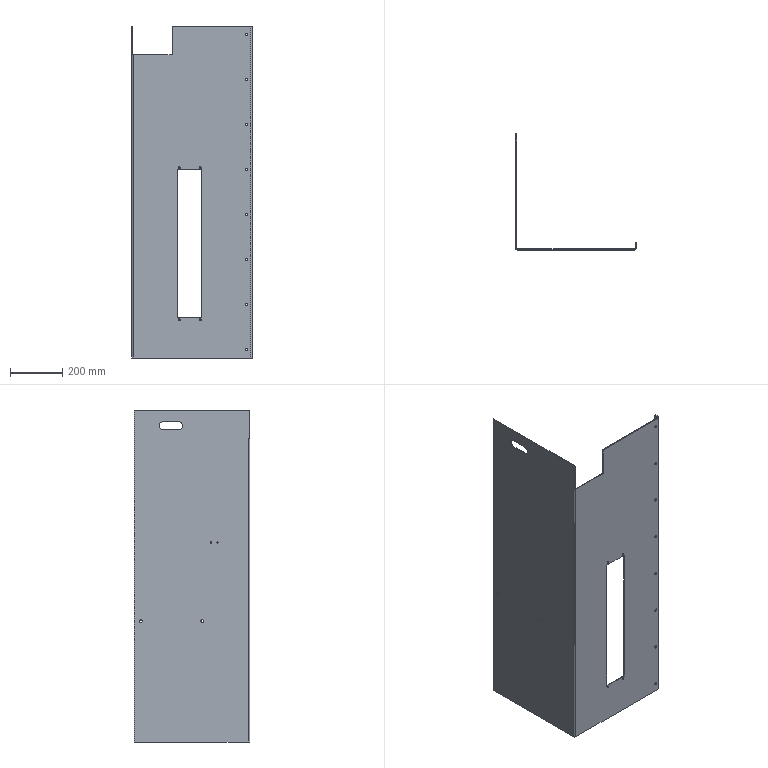Part | NX | features solid 2 | 1 solid | 63 faces | box 458 x 440 x 1265 mm | volume 3246730 mm3 | cylinder 41 | plane 22 | commonest cylinder face diameters 10 x18 8 x8 5.188 x4 10.6 x4 30 x3 6 x2